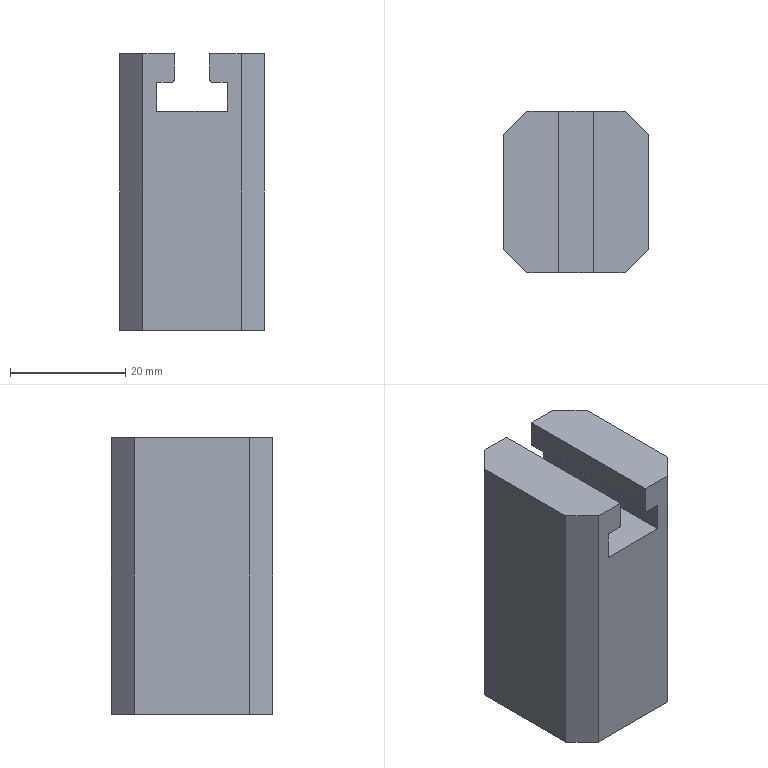Part | Creo | 1 solid | 161 faces | box 25 x 28 x 48 mm | volume 27680 mm3 | other 103 | plane 48 | cylinder 8 | cone 2 | commonest cylinder face diameters 1 x2 8.499 x2 8.5 x2 1.421 x1 22.406 x1